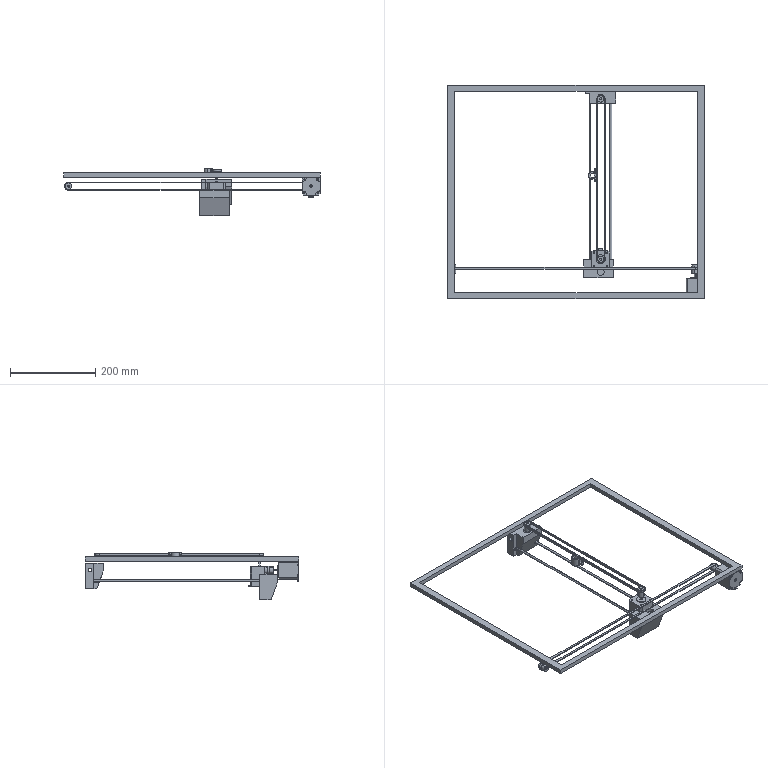Part | SolidWorks | 14 solids | 289 faces | box 600 x 500 x 111.5 mm | volume 820958 mm3 | plane 152 | cylinder 123 | sphere 8 | torus 6 | commonest cylinder face diameters 1 x20 5 x20 3 x16 1.4 x14 15 x14 15.282 x12